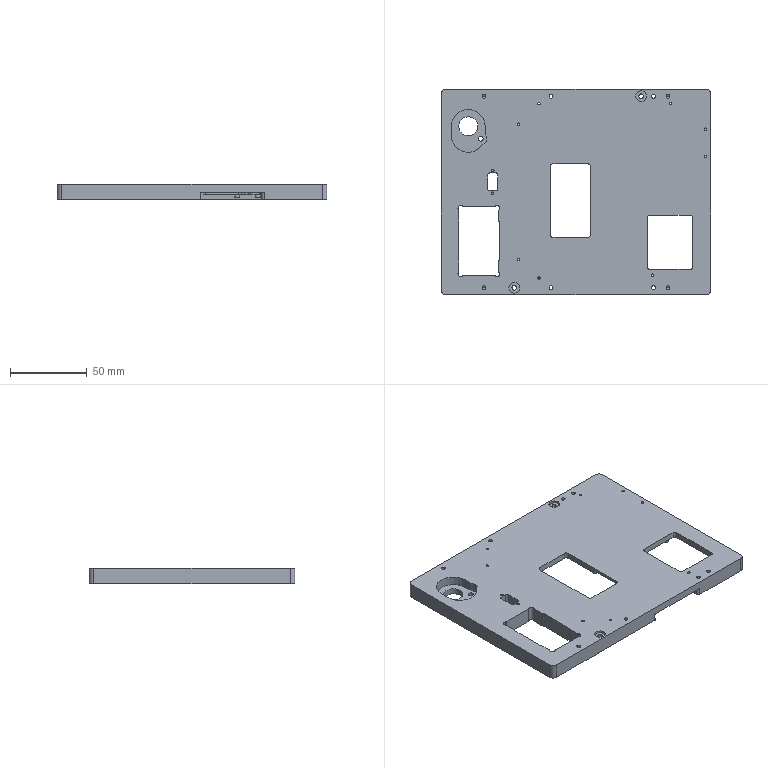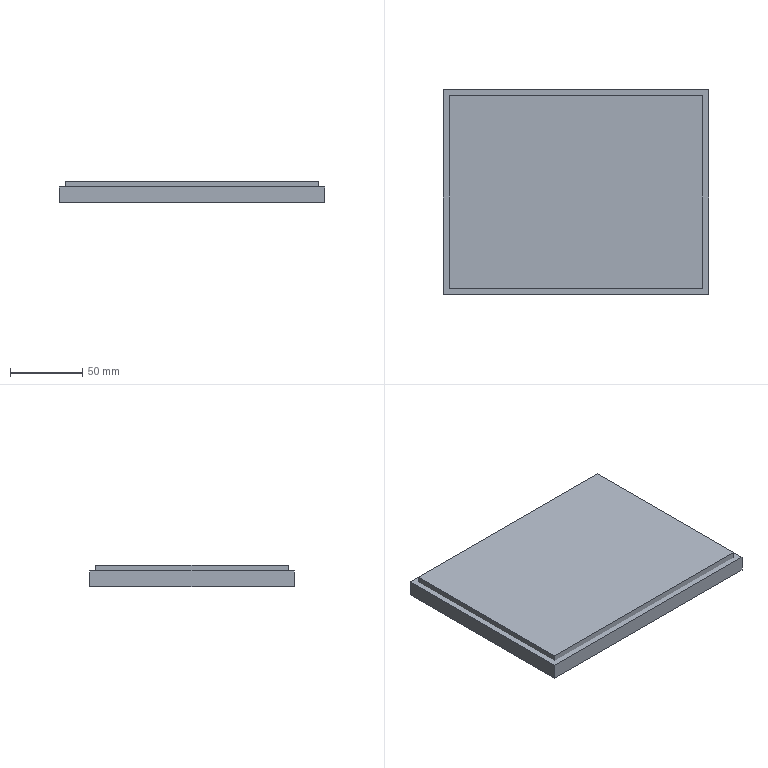CAM job | NX | 3-axis milling, drilling | part box 176 x 134 x 10 mm | stock box 184 x 142 x 15 mm
Tools:
number,name,description,diameter,corner_radius,flute_length,length,flutes
3,D63,Milling Tool-5 Parameters,63.0,0.0,50.0,75.0,2
1,D6A45,Milling Tool-5 Parameters,6.0,0.0,3.0,3.0,2
12,2.5ZT,Drilling Tool,2.5,0.0,35.0,50.0,2
20,1.6ZT,Drilling Tool,1.6,0.0,35.0,50.0,2
23,3.2ZT,Drilling Tool,3.2,0.0,35.0,50.0,2
4,D10,Milling Tool-5 Parameters,10.0,0.0,50.0,75.0,2
13,3.5ZT,Drilling Tool,3.5,0.0,35.0,50.0,2
17,D4,Milling Tool-5 Parameters,4.0,0.0,50.0,75.0,2
16,D6JING,Milling Tool-5 Parameters,6.0,0.0,50.0,75.0,2
19,D2,Milling Tool-5 Parameters,2.0,0.0,50.0,75.0,2
24,D3A45,Milling Tool-5 Parameters,3.0,0.0,1.5,1.5,2
Operations:
program,operation,operation_type,tool,method,geometry_group,spindle_rpm,surface_speed,feed_per_tooth,feed_cut,feed_plunge,cut_length_mm,path_length_mm,cut_time_min,machine_time_min
1,FLOOR_WALL_COPY,VolumeBased25DMillingOperation,D63,METHOD,A,6500.0,1286.0,0.0962,1250.0,100.0,1116.799,1170.799,0.8934,0.8988
1,DRILLING_COPY_1,Operation,D6A45,METHOD,A,5000.0,94.0,0.025,250.0,0.0,91.0,832.788,0.364,0.4382
1,DRILLING_COPY_1_COPY_1,Operation,3.5ZT,METHOD,A,2000.0,21.0,0.0375,150.0,0.0,62.206,284.294,0.4147,0.4369
1,DRILLING_COPY_1_COPY_COPY,Operation,2.5ZT,METHOD,A,2000.0,21.0,0.0375,150.0,0.0,103.209,653.727,0.6881,0.7431
1,DRILLING_COPY_1_COPY,Operation,1.6ZT,METHOD,A,2000.0,21.0,0.025,100.0,0.0,112.607,651.37,1.126,1.18
1,DRILLING_COPY_1_COPY_COPY_COPY,Operation,3.2ZT,METHOD,A,2000.0,21.0,0.0375,150.0,0.0,15.461,90.923,0.1031,0.1106
1,ADAPTIVE_MILLING_COPY,CavityMilling,D10,METHOD,A,9500.0,298.0,0.1842,3500.0,1000.0,5092.449,5298.088,2.018,2.039
1,ZLEVEL_PROFILE_COPY_COPY_COPY_1_COPY_COPY_1_COPY_COPY_COPY_1_COPY_COPY_COPY,ZLevelMilling,D10,METHOD,A,9500.0,298.0,0.1053,2000.0,1000.0,127.417,194.417,0.0876,0.0943
1,ZLEVEL_PROFILE_COPY_COPY_COPY_1_COPY_COPY_1_COPY_COPY_COPY_1_COPY_COPY,ZLevelMilling,D10,METHOD,A,9500.0,298.0,0.1053,2000.0,1000.0,385.65,448.55,0.2167,0.223
1,ZLEVEL_PROFILE_COPY_COPY_COPY_1_COPY_COPY_1_COPY_COPY_COPY_1,ZLevelMilling,D4,METHOD,A,9500.0,89.0,0.0789,1500.0,1000.0,561.214,628.214,0.3862,0.3929
1,ZLEVEL_PROFILE_COPY_COPY_COPY_1_COPY_COPY_1_COPY_COPY_COPY_1_COPY_COPY_COPY_1,ZLevelMilling,D4,METHOD,A,9500.0,89.0,0.0579,1100.0,1000.0,1639.792,3316.776,1.516,1.684
1,FLOOR_WALL,VolumeBased25DMillingOperation,D4,METHOD,A,9500.0,119.0,0.0658,1250.0,100.0,296.017,366.017,0.2368,0.2438
1,ZLEVEL_PROFILE_1_COPY_COPY_COPY_1,ZLevelMilling,D4,METHOD,A,9500.0,298.0,0.0526,1000.0,100.0,792.883,1281.161,0.7929,0.8417
1,HOLE_MILLING,CylinderMilling,D4,METHOD,A,9500.0,119.0,0.0684,1300.0,100.0,154.002,425.936,0.1185,0.1457
1,ZLEVEL_PROFILE_COPY_COPY_COPY_1_COPY_COPY_1_COPY_COPY_COPY_1_COPY_COPY_COPY_COPY,ZLevelMilling,D2,METHOD,A,9500.0,59.0,0.0579,1100.0,1000.0,1726.414,3161.73,1.589,1.733
1,11,ZLevelMilling,D6A45,METHOD,A,9500.0,179.0,0.0526,1000.0,500.0,1306.591,3642.854,1.377,1.611
1,11_COPY_COPY_COPY,ZLevelMilling,D3A45,METHOD,A,9500.0,179.0,0.0526,1000.0,100.0,60.449,208.73,0.0604,0.0753
2,FLOOR_WALL_COPY_COPY,VolumeBased25DMillingOperation,D63,METHOD,B,6500.0,1286.0,0.0962,1250.0,100.0,5383.995,6068.591,4.307,4.376
2,FLOOR_WALL_COPY_COPY_1,VolumeBased25DMillingOperation,D63,METHOD,B,6500.0,1286.0,0.0962,1250.0,100.0,1076.799,1130.799,0.8614,0.8668
2,CAVITY_MILL,CavityMilling,D10,METHOD,B,9500.0,298.0,0.1579,3000.0,1000.0,24204.901,25362.971,8.673,8.789
2,CAVITY_MILL_COPY,CavityMilling,D6JING,METHOD,B,9500.0,179.0,0.0947,1800.0,1000.0,3085.851,9607.16,2.14,2.792
2,CAVITY_MILL_COPY_COPY,CavityMilling,D4,METHOD,B,9500.0,119.0,0.0737,1400.0,1000.0,2878.128,10677.804,2.246,3.026
2,FLOOR_WALL_COPY_1,VolumeBased25DMillingOperation,D4,METHOD,B,9500.0,119.0,0.0658,1250.0,100.0,9133.31,14739.604,7.307,7.867
2,FLOOR_WALL_COPY_1_COPY,VolumeBased25DMillingOperation,D4,METHOD,B,9500.0,119.0,0.0658,1250.0,100.0,1536.169,3251.761,1.229,1.401
2,HOLE_MILLING_COPY,CylinderMilling,D4,METHOD,B,9500.0,119.0,0.0684,1300.0,100.0,148.7,217.4,0.1144,0.1213
2,ZLEVEL_PROFILE_1_COPY_COPY_COPY_1_COPY,ZLevelMilling,D4,METHOD,B,9500.0,298.0,0.0526,1000.0,100.0,253.916,484.532,0.2539,0.277
2,ZLEVEL_PROFILE_1_COPY_COPY_COPY_1_COPY_COPY,ZLevelMilling,D4,METHOD,B,9500.0,298.0,0.0526,1000.0,100.0,103.547,167.747,0.1035,0.11
2,ZLEVEL_PROFILE_COPY_COPY_COPY_1_COPY_COPY_1_COPY_COPY_COPY_1_COPY_COPY_COPY_COPY_1,ZLevelMilling,D2,METHOD,B,9500.0,59.0,0.0579,1100.0,1000.0,2894.685,11448.927,2.673,3.529
2,FLOOR_WALL_COPY_1_COPY_1,VolumeBased25DMillingOperation,D2,METHOD,B,9500.0,59.0,0.0526,1000.0,100.0,242.872,767.181,0.2429,0.2953
2,11_COPY,ZLevelMilling,D6A45,METHOD,B,9500.0,179.0,0.0526,1000.0,500.0,1189.465,2836.164,1.244,1.408
2,11_COPY_COPY,ZLevelMilling,D6A45,METHOD,B,9500.0,179.0,0.0526,1000.0,500.0,790.846,2254.197,0.8448,0.9911
2,11_COPY_COPY_COPY_COPY,ZLevelMilling,D6A45,METHOD,B,9500.0,179.0,0.0526,1000.0,500.0,407.717,1300.899,0.4462,0.5355
2,刀补17,ZLevelMilling,D4,METHOD,B,9500.0,298.0,0.0526,1000.0,100.0,107.645,501.473,0.1076,0.147